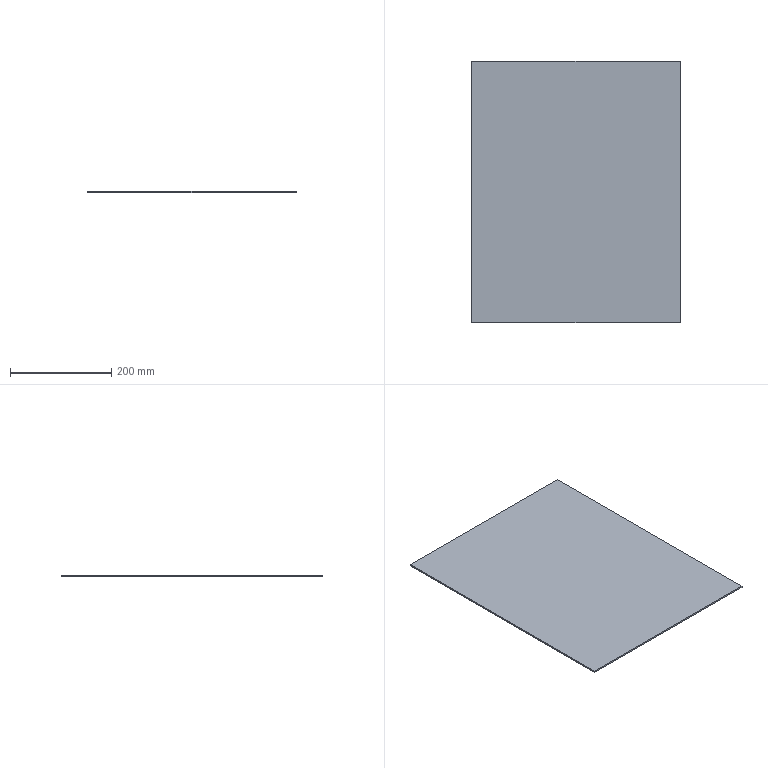Part | STEP file | x77-05403 | 1 solid | 6 faces | box 411 x 515 x 3 mm | volume 634995 mm3 | plane 6
STEP:
#1=CARTESIAN_POINT('',(206.8,258.8,0.));
#2=VERTEX_POINT('',#1);
#3=CARTESIAN_POINT('',(-204.2,258.8,0.));
#4=VERTEX_POINT('',#3);
#5=CARTESIAN_POINT('',(-204.2,258.8,0.));
#6=DIRECTION('',(-1.,0.,0.));
#7=VECTOR('',#6,1000.);
#8=LINE('',#5,#7);
#9=EDGE_CURVE('',#2,#4,#8,.T.);
#10=ORIENTED_EDGE('',*,*,#9,.T.);
#11=CARTESIAN_POINT('',(-204.2,258.8,3.));
#12=VERTEX_POINT('',#11);
#13=CARTESIAN_POINT('',(-204.2,258.8,3.));
#14=DIRECTION('',(0.,0.,-1.));
#15=VECTOR('',#14,1000.);
#16=LINE('',#13,#15);
#17=EDGE_CURVE('',#12,#4,#16,.T.);
#18=ORIENTED_EDGE('',*,*,#17,.F.);
#19=CARTESIAN_POINT('',(206.8,258.8,3.));
#20=VERTEX_POINT('',#19);
#21=CARTESIAN_POINT('',(-204.2,258.8,3.));
#22=DIRECTION('',(-1.,0.,0.));
#23=VECTOR('',#22,1000.);
#24=LINE('',#21,#23);
#25=EDGE_CURVE('',#20,#12,#24,.T.);
#26=ORIENTED_EDGE('',*,*,#25,.F.);
#27=CARTESIAN_POINT('',(206.8,258.8,3.));
#28=DIRECTION('',(0.,0.,-1.));
#29=VECTOR('',#28,1000.);
#30=LINE('',#27,#29);
#31=EDGE_CURVE('',#20,#2,#30,.T.);
#32=ORIENTED_EDGE('',*,*,#31,.T.);
#33=EDGE_LOOP('',(#10,#18,#26,#32));
#34=FACE_OUTER_BOUND('',#33,.T.);
#35=CARTESIAN_POINT('',(-204.2,258.8,3.));
#36=DIRECTION('',(0.,-1.,0.));
#37=DIRECTION('',(0.,0.,-1.));
#38=AXIS2_PLACEMENT_3D('',#35,#36,#37);
#39=PLANE('',#38);
#40=ADVANCED_FACE('',(#34),#39,.F.);
#41=CARTESIAN_POINT('',(-204.2,-256.2,0.));
#42=VERTEX_POINT('',#41);
#43=CARTESIAN_POINT('',(-204.2,258.8,0.));
#44=DIRECTION('',(0.,-1.,0.));
#45=VECTOR('',#44,1000.);
#46=LINE('',#43,#45);
#47=EDGE_CURVE('',#4,#42,#46,.T.);
#48=ORIENTED_EDGE('',*,*,#47,.T.);
#49=CARTESIAN_POINT('',(-204.2,-256.2,3.));
#50=VERTEX_POINT('',#49);
#51=CARTESIAN_POINT('',(-204.2,-256.2,3.));
#52=DIRECTION('',(0.,0.,-1.));
#53=VECTOR('',#52,1000.);
#54=LINE('',#51,#53);
#55=EDGE_CURVE('',#50,#42,#54,.T.);
#56=ORIENTED_EDGE('',*,*,#55,.F.);
#57=CARTESIAN_POINT('',(-204.2,258.8,3.));
#58=DIRECTION('',(0.,-1.,0.));
#59=VECTOR('',#58,1000.);
#60=LINE('',#57,#59);
#61=EDGE_CURVE('',#12,#50,#60,.T.);
#62=ORIENTED_EDGE('',*,*,#61,.F.);
#63=ORIENTED_EDGE('',*,*,#17,.T.);
#64=EDGE_LOOP('',(#48,#56,#62,#63));
#65=FACE_OUTER_BOUND('',#64,.T.);
#66=CARTESIAN_POINT('',(-204.2,258.8,3.));
#67=DIRECTION('',(1.,0.,0.));
#68=DIRECTION('',(0.,0.,-1.));
#69=AXIS2_PLACEMENT_3D('',#66,#67,#68);
#70=PLANE('',#69);
#71=ADVANCED_FACE('',(#65),#70,.F.);
#72=CARTESIAN_POINT('',(206.8,-256.2,0.));
#73=VERTEX_POINT('',#72);
#74=CARTESIAN_POINT('',(-204.2,-256.2,0.));
#75=DIRECTION('',(1.,0.,0.));
#76=VECTOR('',#75,1000.);
#77=LINE('',#74,#76);
#78=EDGE_CURVE('',#42,#73,#77,.T.);
#79=ORIENTED_EDGE('',*,*,#78,.T.);
#80=CARTESIAN_POINT('',(206.8,-256.2,3.));
#81=VERTEX_POINT('',#80);
#82=CARTESIAN_POINT('',(206.8,-256.2,3.));
#83=DIRECTION('',(0.,0.,-1.));
#84=VECTOR('',#83,1000.);
#85=LINE('',#82,#84);
#86=EDGE_CURVE('',#81,#73,#85,.T.);
#87=ORIENTED_EDGE('',*,*,#86,.F.);
#88=CARTESIAN_POINT('',(-204.2,-256.2,3.));
#89=DIRECTION('',(1.,0.,0.));
#90=VECTOR('',#89,1000.);
#91=LINE('',#88,#90);
#92=EDGE_CURVE('',#50,#81,#91,.T.);
#93=ORIENTED_EDGE('',*,*,#92,.F.);
#94=ORIENTED_EDGE('',*,*,#55,.T.);
#95=EDGE_LOOP('',(#79,#87,#93,#94));
#96=FACE_OUTER_BOUND('',#95,.T.);
#97=CARTESIAN_POINT('',(-204.2,-256.2,3.));
#98=DIRECTION('',(0.,1.,0.));
#99=DIRECTION('',(-1.,0.,0.));
#100=AXIS2_PLACEMENT_3D('',#97,#98,#99);
#101=PLANE('',#100);
#102=ADVANCED_FACE('',(#96),#101,.F.);
#103=CARTESIAN_POINT('',(206.8,258.8,0.));
#104=DIRECTION('',(0.,1.,0.));
#105=VECTOR('',#104,1000.);
#106=LINE('',#103,#105);
#107=EDGE_CURVE('',#73,#2,#106,.T.);
#108=ORIENTED_EDGE('',*,*,#107,.T.);
#109=ORIENTED_EDGE('',*,*,#31,.F.);
#110=CARTESIAN_POINT('',(206.8,258.8,3.));
#111=DIRECTION('',(0.,1.,0.));
#112=VECTOR('',#111,1000.);
#113=LINE('',#110,#112);
#114=EDGE_CURVE('',#81,#20,#113,.T.);
#115=ORIENTED_EDGE('',*,*,#114,.F.);
#116=ORIENTED_EDGE('',*,*,#86,.T.);
#117=EDGE_LOOP('',(#108,#109,#115,#116));
#118=FACE_OUTER_BOUND('',#117,.T.);
#119=CARTESIAN_POINT('',(206.8,258.8,3.));
#120=DIRECTION('',(-1.,0.,0.));
#121=DIRECTION('',(0.,0.,1.));
#122=AXIS2_PLACEMENT_3D('',#119,#120,#121);
#123=PLANE('',#122);
#124=ADVANCED_FACE('',(#118),#123,.F.);
#125=ORIENTED_EDGE('',*,*,#25,.T.);
#126=ORIENTED_EDGE('',*,*,#61,.T.);
#127=ORIENTED_EDGE('',*,*,#92,.T.);
#128=ORIENTED_EDGE('',*,*,#114,.T.);
#129=EDGE_LOOP('',(#125,#126,#127,#128));
#130=FACE_OUTER_BOUND('',#129,.T.);
#131=CARTESIAN_POINT('',(206.8,258.8,3.));
#132=DIRECTION('',(0.,0.,-1.));
#133=DIRECTION('',(-1.,0.,0.));
#134=AXIS2_PLACEMENT_3D('',#131,#132,#133);
#135=PLANE('',#134);
#136=ADVANCED_FACE('',(#130),#135,.F.);
#137=ORIENTED_EDGE('',*,*,#9,.F.);
#138=ORIENTED_EDGE('',*,*,#107,.F.);
#139=ORIENTED_EDGE('',*,*,#78,.F.);
#140=ORIENTED_EDGE('',*,*,#47,.F.);
#141=EDGE_LOOP('',(#137,#138,#139,#140));
#142=FACE_OUTER_BOUND('',#141,.T.);
#143=CARTESIAN_POINT('',(206.8,258.8,0.));
#144=DIRECTION('',(0.,0.,-1.));
#145=DIRECTION('',(-1.,0.,0.));
#146=AXIS2_PLACEMENT_3D('',#143,#144,#145);
#147=PLANE('',#146);
#148=ADVANCED_FACE('',(#142),#147,.T.);
#149=CLOSED_SHELL('',(#40,#71,#102,#124,#136,#148));
#150=MANIFOLD_SOLID_BREP('',#149);
#151=CARTESIAN_POINT('',(0.,0.,0.));
#152=DIRECTION('',(0.,0.,1.));
#153=DIRECTION('',(1.,0.,0.));
#154=AXIS2_PLACEMENT_3D('',#151,#152,#153);
#155=(LENGTH_UNIT()NAMED_UNIT(*)SI_UNIT(.MILLI.,.METRE.));
#156=UNCERTAINTY_MEASURE_WITH_UNIT(LENGTH_MEASURE(0.00001),#155,'','');
#157=(NAMED_UNIT(*)PLANE_ANGLE_UNIT()SI_UNIT($,.RADIAN.));
#158=(NAMED_UNIT(*)SI_UNIT($,.STERADIAN.)SOLID_ANGLE_UNIT());
#159=(GEOMETRIC_REPRESENTATION_CONTEXT(3)GLOBAL_UNCERTAINTY_ASSIGNED_CONTEXT((#156))GLOBAL_UNIT_ASSIGNED_CONTEXT((#155,#157,#158))REPRESENTATION_CONTEXT('',''));
#160=ADVANCED_BREP_SHAPE_REPRESENTATION('',(#150,#154),#159);